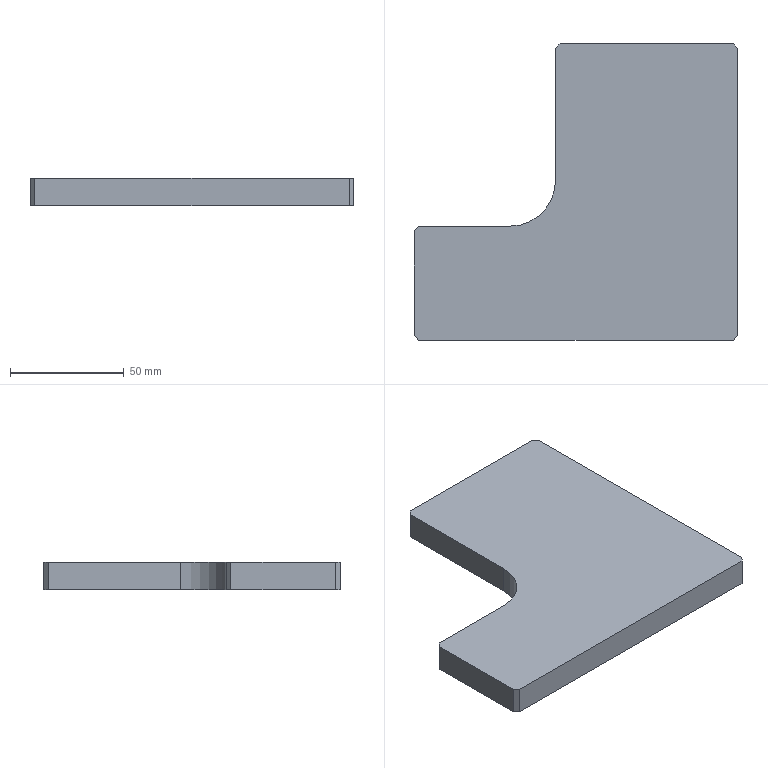Part | STEP file | 001-005-Shaft threading fixture cylinder mounting plate | 1 solid | 18 faces | box 142 x 130 x 12 mm | volume 162627 mm3 | plane 13 | cylinder 3 | cone 2 | commonest cylinder face diameters 4.2 x2 40 x1
STEP:
#1=CARTESIAN_POINT('',(0.,0.,0.));
#2=DIRECTION('',(0.,0.,1.));
#3=DIRECTION('',(1.,0.,0.));
#4=AXIS2_PLACEMENT_3D('',#1,#2,#3);
#5=CARTESIAN_POINT('',(31.,45.,8.1));
#6=VERTEX_POINT('',#5);
#7=CARTESIAN_POINT('',(31.,65.,8.1));
#8=VERTEX_POINT('',#7);
#9=CARTESIAN_POINT('',(31.,65.,8.1));
#10=DIRECTION('',(0.,1.,0.));
#11=VECTOR('',#10,1.);
#12=LINE('',#9,#11);
#13=CARTESIAN_POINT('',(31.,65.,6.));
#14=DIRECTION('',(0.,1.,0.));
#15=DIRECTION('',(0.,0.,1.));
#16=AXIS2_PLACEMENT_3D('',#13,#14,#15);
#17=CYLINDRICAL_SURFACE('',#16,2.1);
#18=CARTESIAN_POINT('',(6.283,0.));
#19=DIRECTION('',(0.,1.));
#20=VECTOR('',#19,1.);
#21=LINE('',#18,#20);
#22=(GEOMETRIC_REPRESENTATION_CONTEXT(2)PARAMETRIC_REPRESENTATION_CONTEXT()REPRESENTATION_CONTEXT('',''));
#23=DEFINITIONAL_REPRESENTATION('',(#21),#22);
#24=PCURVE('',#17,#23);
#25=CARTESIAN_POINT('',(31.,65.,6.));
#26=DIRECTION('',(0.,1.,0.));
#27=DIRECTION('',(0.,0.,1.));
#28=AXIS2_PLACEMENT_3D('',#25,#26,#27);
#29=CYLINDRICAL_SURFACE('',#28,2.1);
#30=CARTESIAN_POINT('',(0.,0.));
#31=DIRECTION('',(0.,1.));
#32=VECTOR('',#31,1.);
#33=LINE('',#30,#32);
#34=(GEOMETRIC_REPRESENTATION_CONTEXT(2)PARAMETRIC_REPRESENTATION_CONTEXT()REPRESENTATION_CONTEXT('',''));
#35=DEFINITIONAL_REPRESENTATION('',(#33),#34);
#36=PCURVE('',#29,#35);
#37=SURFACE_CURVE('',#12,(#24,#36),.PCURVE_S1.);
#38=EDGE_CURVE('',#6,#8,#37,.T.);
#39=ORIENTED_EDGE('',*,*,#38,.T.);
#40=CARTESIAN_POINT('',(31.,65.,3.9));
#41=VERTEX_POINT('',#40);
#42=CARTESIAN_POINT('',(31.,65.,6.));
#43=DIRECTION('',(0.,1.,0.));
#44=DIRECTION('',(0.,0.,1.));
#45=AXIS2_PLACEMENT_3D('',#42,#43,#44);
#46=CIRCLE('',#45,2.1);
#47=CARTESIAN_POINT('',(0.,0.));
#48=DIRECTION('',(1.,0.));
#49=VECTOR('',#48,1.);
#50=LINE('',#47,#49);
#51=(GEOMETRIC_REPRESENTATION_CONTEXT(2)PARAMETRIC_REPRESENTATION_CONTEXT()REPRESENTATION_CONTEXT('',''));
#52=DEFINITIONAL_REPRESENTATION('',(#50),#51);
#53=PCURVE('',#17,#52);
#54=CARTESIAN_POINT('',(-71.,65.,12.));
#55=DIRECTION('',(0.,-1.,0.));
#56=DIRECTION('',(1.,0.,0.));
#57=AXIS2_PLACEMENT_3D('',#54,#55,#56);
#58=PLANE('',#57);
#59=CARTESIAN_POINT('',(102.,-3.9));
#60=CARTESIAN_POINT('',(105.637,-3.9));
#61=CARTESIAN_POINT('',(103.819,-7.05));
#62=CARTESIAN_POINT('',(102.,-10.2));
#63=CARTESIAN_POINT('',(100.181,-7.05));
#64=CARTESIAN_POINT('',(98.363,-3.9));
#65=CARTESIAN_POINT('',(102.,-3.9));
#66=(BOUNDED_CURVE()B_SPLINE_CURVE(2,(#59,#60,#61,#62,#63,#64,#65),.UNSPECIFIED.,.T.,.F.)B_SPLINE_CURVE_WITH_KNOTS((1,2,2,2,2,1),(-2.094,0.,2.094,4.189,6.283,8.378),.UNSPECIFIED.)CURVE()GEOMETRIC_REPRESENTATION_ITEM()RATIONAL_B_SPLINE_CURVE((1.,0.5,1.,0.5,1.,0.5,1.))REPRESENTATION_ITEM(''));
#67=(GEOMETRIC_REPRESENTATION_CONTEXT(2)PARAMETRIC_REPRESENTATION_CONTEXT()REPRESENTATION_CONTEXT('',''));
#68=DEFINITIONAL_REPRESENTATION('',(#66),#67);
#69=PCURVE('',#58,#68);
#70=SURFACE_CURVE('',#46,(#53,#69),.PCURVE_S1.);
#71=EDGE_CURVE('',#41,#8,#70,.T.);
#72=ORIENTED_EDGE('',*,*,#71,.F.);
#73=CARTESIAN_POINT('',(31.,45.,3.9));
#74=VERTEX_POINT('',#73);
#75=CARTESIAN_POINT('',(31.,65.,3.9));
#76=DIRECTION('',(0.,1.,0.));
#77=VECTOR('',#76,1.);
#78=LINE('',#75,#77);
#79=CARTESIAN_POINT('',(3.142,0.));
#80=DIRECTION('',(0.,1.));
#81=VECTOR('',#80,1.);
#82=LINE('',#79,#81);
#83=(GEOMETRIC_REPRESENTATION_CONTEXT(2)PARAMETRIC_REPRESENTATION_CONTEXT()REPRESENTATION_CONTEXT('',''));
#84=DEFINITIONAL_REPRESENTATION('',(#82),#83);
#85=PCURVE('',#17,#84);
#86=CARTESIAN_POINT('',(3.142,0.));
#87=DIRECTION('',(0.,1.));
#88=VECTOR('',#87,1.);
#89=LINE('',#86,#88);
#90=(GEOMETRIC_REPRESENTATION_CONTEXT(2)PARAMETRIC_REPRESENTATION_CONTEXT()REPRESENTATION_CONTEXT('',''));
#91=DEFINITIONAL_REPRESENTATION('',(#89),#90);
#92=PCURVE('',#29,#91);
#93=SURFACE_CURVE('',#78,(#85,#92),.PCURVE_S1.);
#94=EDGE_CURVE('',#74,#41,#93,.T.);
#95=ORIENTED_EDGE('',*,*,#94,.F.);
#96=CARTESIAN_POINT('',(31.,45.,6.));
#97=DIRECTION('',(0.,1.,0.));
#98=DIRECTION('',(0.,0.,1.));
#99=AXIS2_PLACEMENT_3D('',#96,#97,#98);
#100=CIRCLE('',#99,2.1);
#101=CARTESIAN_POINT('',(0.,-20.));
#102=DIRECTION('',(1.,0.));
#103=VECTOR('',#102,1.);
#104=LINE('',#101,#103);
#105=(GEOMETRIC_REPRESENTATION_CONTEXT(2)PARAMETRIC_REPRESENTATION_CONTEXT()REPRESENTATION_CONTEXT('',''));
#106=DEFINITIONAL_REPRESENTATION('',(#104),#105);
#107=PCURVE('',#17,#106);
#108=CARTESIAN_POINT('',(31.,45.,6.));
#109=DIRECTION('',(0.,1.,0.));
#110=DIRECTION('',(0.,0.,1.));
#111=AXIS2_PLACEMENT_3D('',#108,#109,#110);
#112=CONICAL_SURFACE('',#111,2.1,1.03);
#113=CARTESIAN_POINT('',(0.,0.));
#114=DIRECTION('',(1.,0.));
#115=VECTOR('',#114,1.);
#116=LINE('',#113,#115);
#117=(GEOMETRIC_REPRESENTATION_CONTEXT(2)PARAMETRIC_REPRESENTATION_CONTEXT()REPRESENTATION_CONTEXT('',''));
#118=DEFINITIONAL_REPRESENTATION('',(#116),#117);
#119=PCURVE('',#112,#118);
#120=SURFACE_CURVE('',#100,(#107,#119),.PCURVE_S1.);
#121=EDGE_CURVE('',#74,#6,#120,.T.);
#122=ORIENTED_EDGE('',*,*,#121,.T.);
#123=EDGE_LOOP('',(#39,#72,#95,#122));
#124=FACE_BOUND('',#123,.F.);
#125=ADVANCED_FACE('',(#124),#17,.F.);
#126=ORIENTED_EDGE('',*,*,#121,.F.);
#127=CARTESIAN_POINT('',(31.,43.738,6.));
#128=VERTEX_POINT('',#127);
#129=CARTESIAN_POINT('',(31.,45.,3.9));
#130=DIRECTION('',(0.,0.515,-0.8572));
#131=VECTOR('',#130,1.);
#132=LINE('',#129,#131);
#133=CARTESIAN_POINT('',(3.142,-1.262));
#134=CARTESIAN_POINT('',(3.142,-1.243));
#135=CARTESIAN_POINT('',(3.142,-1.204));
#136=CARTESIAN_POINT('',(3.142,-1.147));
#137=CARTESIAN_POINT('',(3.142,-1.09));
#138=CARTESIAN_POINT('',(3.142,-1.032));
#139=CARTESIAN_POINT('',(3.142,-0.975));
#140=CARTESIAN_POINT('',(3.142,-0.9177));
#141=CARTESIAN_POINT('',(3.142,-0.8603));
#142=CARTESIAN_POINT('',(3.142,-0.803));
#143=CARTESIAN_POINT('',(3.142,-0.7456));
#144=CARTESIAN_POINT('',(3.142,-0.6883));
#145=CARTESIAN_POINT('',(3.142,-0.6309));
#146=CARTESIAN_POINT('',(3.142,-0.5735));
#147=CARTESIAN_POINT('',(3.142,-0.5162));
#148=CARTESIAN_POINT('',(3.142,-0.4588));
#149=CARTESIAN_POINT('',(3.142,-0.4015));
#150=CARTESIAN_POINT('',(3.142,-0.3441));
#151=CARTESIAN_POINT('',(3.142,-0.2868));
#152=CARTESIAN_POINT('',(3.142,-0.2294));
#153=CARTESIAN_POINT('',(3.142,-0.1721));
#154=CARTESIAN_POINT('',(3.142,-0.1147));
#155=CARTESIAN_POINT('',(3.142,-0.05735));
#156=CARTESIAN_POINT('',(3.142,-0.01912));
#157=CARTESIAN_POINT('',(3.142,0.));
#158=B_SPLINE_CURVE_WITH_KNOTS('',3,(#133,#134,#135,#136,#137,#138,#139,#140,#141,#142,#143,#144,#145,#146,#147,#148,#149,#150,#151,#152,#153,#154,#155,#156,#157),.UNSPECIFIED.,.F.,.F.,(4,1,1,1,1,1,1,1,1,1,1,1,1,1,1,1,1,1,1,1,1,1,4),(-2.45,-2.339,-2.227,-2.116,-2.004,-1.893,-1.782,-1.67,-1.559,-1.448,-1.336,-1.225,-1.114,-1.002,-0.8909,-0.7795,-0.6682,-0.5568,-0.4454,-0.3341,-0.2227,-0.1114,0.),.QUASI_UNIFORM_KNOTS.);
#159=(GEOMETRIC_REPRESENTATION_CONTEXT(2)PARAMETRIC_REPRESENTATION_CONTEXT()REPRESENTATION_CONTEXT('',''));
#160=DEFINITIONAL_REPRESENTATION('',(#158),#159);
#161=PCURVE('',#112,#160);
#162=CARTESIAN_POINT('',(31.,45.,6.));
#163=DIRECTION('',(0.,1.,0.));
#164=DIRECTION('',(0.,0.,1.));
#165=AXIS2_PLACEMENT_3D('',#162,#163,#164);
#166=CONICAL_SURFACE('',#165,2.1,1.03);
#167=CARTESIAN_POINT('',(3.142,-1.262));
#168=CARTESIAN_POINT('',(3.142,-1.243));
#169=CARTESIAN_POINT('',(3.142,-1.204));
#170=CARTESIAN_POINT('',(3.142,-1.147));
#171=CARTESIAN_POINT('',(3.142,-1.09));
#172=CARTESIAN_POINT('',(3.142,-1.032));
#173=CARTESIAN_POINT('',(3.142,-0.975));
#174=CARTESIAN_POINT('',(3.142,-0.9177));
#175=CARTESIAN_POINT('',(3.142,-0.8603));
#176=CARTESIAN_POINT('',(3.142,-0.803));
#177=CARTESIAN_POINT('',(3.142,-0.7456));
#178=CARTESIAN_POINT('',(3.142,-0.6883));
#179=CARTESIAN_POINT('',(3.142,-0.6309));
#180=CARTESIAN_POINT('',(3.142,-0.5735));
#181=CARTESIAN_POINT('',(3.142,-0.5162));
#182=CARTESIAN_POINT('',(3.142,-0.4588));
#183=CARTESIAN_POINT('',(3.142,-0.4015));
#184=CARTESIAN_POINT('',(3.142,-0.3441));
#185=CARTESIAN_POINT('',(3.142,-0.2868));
#186=CARTESIAN_POINT('',(3.142,-0.2294));
#187=CARTESIAN_POINT('',(3.142,-0.1721));
#188=CARTESIAN_POINT('',(3.142,-0.1147));
#189=CARTESIAN_POINT('',(3.142,-0.05735));
#190=CARTESIAN_POINT('',(3.142,-0.01912));
#191=CARTESIAN_POINT('',(3.142,0.));
#192=B_SPLINE_CURVE_WITH_KNOTS('',3,(#167,#168,#169,#170,#171,#172,#173,#174,#175,#176,#177,#178,#179,#180,#181,#182,#183,#184,#185,#186,#187,#188,#189,#190,#191),.UNSPECIFIED.,.F.,.F.,(4,1,1,1,1,1,1,1,1,1,1,1,1,1,1,1,1,1,1,1,1,1,4),(-2.45,-2.339,-2.227,-2.116,-2.004,-1.893,-1.782,-1.67,-1.559,-1.448,-1.336,-1.225,-1.114,-1.002,-0.8909,-0.7795,-0.6682,-0.5568,-0.4454,-0.3341,-0.2227,-0.1114,0.),.QUASI_UNIFORM_KNOTS.);
#193=(GEOMETRIC_REPRESENTATION_CONTEXT(2)PARAMETRIC_REPRESENTATION_CONTEXT()REPRESENTATION_CONTEXT('',''));
#194=DEFINITIONAL_REPRESENTATION('',(#192),#193);
#195=PCURVE('',#166,#194);
#196=SURFACE_CURVE('',#132,(#161,#195),.PCURVE_S1.);
#197=EDGE_CURVE('',#128,#74,#196,.T.);
#198=ORIENTED_EDGE('',*,*,#197,.F.);
#199=CARTESIAN_POINT('',(31.,45.,8.1));
#200=DIRECTION('',(0.,0.515,0.8572));
#201=VECTOR('',#200,1.);
#202=LINE('',#199,#201);
#203=CARTESIAN_POINT('',(6.283,-1.262));
#204=CARTESIAN_POINT('',(6.283,-1.243));
#205=CARTESIAN_POINT('',(6.283,-1.204));
#206=CARTESIAN_POINT('',(6.283,-1.147));
#207=CARTESIAN_POINT('',(6.283,-1.09));
#208=CARTESIAN_POINT('',(6.283,-1.032));
#209=CARTESIAN_POINT('',(6.283,-0.975));
#210=CARTESIAN_POINT('',(6.283,-0.9177));
#211=CARTESIAN_POINT('',(6.283,-0.8603));
#212=CARTESIAN_POINT('',(6.283,-0.803));
#213=CARTESIAN_POINT('',(6.283,-0.7456));
#214=CARTESIAN_POINT('',(6.283,-0.6883));
#215=CARTESIAN_POINT('',(6.283,-0.6309));
#216=CARTESIAN_POINT('',(6.283,-0.5735));
#217=CARTESIAN_POINT('',(6.283,-0.5162));
#218=CARTESIAN_POINT('',(6.283,-0.4588));
#219=CARTESIAN_POINT('',(6.283,-0.4015));
#220=CARTESIAN_POINT('',(6.283,-0.3441));
#221=CARTESIAN_POINT('',(6.283,-0.2868));
#222=CARTESIAN_POINT('',(6.283,-0.2294));
#223=CARTESIAN_POINT('',(6.283,-0.1721));
#224=CARTESIAN_POINT('',(6.283,-0.1147));
#225=CARTESIAN_POINT('',(6.283,-0.05735));
#226=CARTESIAN_POINT('',(6.283,-0.01912));
#227=CARTESIAN_POINT('',(6.283,0.));
#228=B_SPLINE_CURVE_WITH_KNOTS('',3,(#203,#204,#205,#206,#207,#208,#209,#210,#211,#212,#213,#214,#215,#216,#217,#218,#219,#220,#221,#222,#223,#224,#225,#226,#227),.UNSPECIFIED.,.F.,.F.,(4,1,1,1,1,1,1,1,1,1,1,1,1,1,1,1,1,1,1,1,1,1,4),(-2.45,-2.339,-2.227,-2.116,-2.004,-1.893,-1.782,-1.67,-1.559,-1.448,-1.336,-1.225,-1.114,-1.002,-0.8909,-0.7795,-0.6682,-0.5568,-0.4454,-0.3341,-0.2227,-0.1114,0.),.UNSPECIFIED.);
#229=(GEOMETRIC_REPRESENTATION_CONTEXT(2)PARAMETRIC_REPRESENTATION_CONTEXT()REPRESENTATION_CONTEXT('',''));
#230=DEFINITIONAL_REPRESENTATION('',(#228),#229);
#231=PCURVE('',#112,#230);
#232=CARTESIAN_POINT('',(0.,-1.262));
#233=CARTESIAN_POINT('',(0.,-1.243));
#234=CARTESIAN_POINT('',(0.,-1.204));
#235=CARTESIAN_POINT('',(0.,-1.147));
#236=CARTESIAN_POINT('',(0.,-1.09));
#237=CARTESIAN_POINT('',(0.,-1.032));
#238=CARTESIAN_POINT('',(0.,-0.975));
#239=CARTESIAN_POINT('',(0.,-0.9177));
#240=CARTESIAN_POINT('',(0.,-0.8603));
#241=CARTESIAN_POINT('',(0.,-0.803));
#242=CARTESIAN_POINT('',(0.,-0.7456));
#243=CARTESIAN_POINT('',(0.,-0.6883));
#244=CARTESIAN_POINT('',(0.,-0.6309));
#245=CARTESIAN_POINT('',(0.,-0.5735));
#246=CARTESIAN_POINT('',(0.,-0.5162));
#247=CARTESIAN_POINT('',(0.,-0.4588));
#248=CARTESIAN_POINT('',(0.,-0.4015));
#249=CARTESIAN_POINT('',(0.,-0.3441));
#250=CARTESIAN_POINT('',(0.,-0.2868));
#251=CARTESIAN_POINT('',(0.,-0.2294));
#252=CARTESIAN_POINT('',(0.,-0.1721));
#253=CARTESIAN_POINT('',(0.,-0.1147));
#254=CARTESIAN_POINT('',(0.,-0.05735));
#255=CARTESIAN_POINT('',(0.,-0.01912));
#256=CARTESIAN_POINT('',(0.,0.));
#257=B_SPLINE_CURVE_WITH_KNOTS('',3,(#232,#233,#234,#235,#236,#237,#238,#239,#240,#241,#242,#243,#244,#245,#246,#247,#248,#249,#250,#251,#252,#253,#254,#255,#256),.UNSPECIFIED.,.F.,.F.,(4,1,1,1,1,1,1,1,1,1,1,1,1,1,1,1,1,1,1,1,1,1,4),(-2.45,-2.339,-2.227,-2.116,-2.004,-1.893,-1.782,-1.67,-1.559,-1.448,-1.336,-1.225,-1.114,-1.002,-0.8909,-0.7795,-0.6682,-0.5568,-0.4454,-0.3341,-0.2227,-0.1114,0.),.UNSPECIFIED.);
#258=(GEOMETRIC_REPRESENTATION_CONTEXT(2)PARAMETRIC_REPRESENTATION_CONTEXT()REPRESENTATION_CONTEXT('',''));
#259=DEFINITIONAL_REPRESENTATION('',(#257),#258);
#260=PCURVE('',#166,#259);
#261=SURFACE_CURVE('',#202,(#231,#260),.PCURVE_S1.);
#262=EDGE_CURVE('',#128,#6,#261,.T.);
#263=ORIENTED_EDGE('',*,*,#262,.T.);
#264=EDGE_LOOP('',(#126,#198,#263));
#265=FACE_BOUND('',#264,.F.);
#266=ADVANCED_FACE('',(#265),#112,.F.);
#267=CARTESIAN_POINT('',(31.,65.,6.));
#268=DIRECTION('',(0.,1.,0.));
#269=DIRECTION('',(0.,0.,1.));
#270=AXIS2_PLACEMENT_3D('',#267,#268,#269);
#271=CIRCLE('',#270,2.1);
#272=CARTESIAN_POINT('',(102.,-3.9));
#273=CARTESIAN_POINT('',(105.637,-3.9));
#274=CARTESIAN_POINT('',(103.819,-7.05));
#275=CARTESIAN_POINT('',(102.,-10.2));
#276=CARTESIAN_POINT('',(100.181,-7.05));
#277=CARTESIAN_POINT('',(98.363,-3.9));
#278=CARTESIAN_POINT('',(102.,-3.9));
#279=(BOUNDED_CURVE()B_SPLINE_CURVE(2,(#272,#273,#274,#275,#276,#277,#278),.UNSPECIFIED.,.T.,.F.)B_SPLINE_CURVE_WITH_KNOTS((1,2,2,2,2,1),(-2.094,0.,2.094,4.189,6.283,8.378),.UNSPECIFIED.)CURVE()GEOMETRIC_REPRESENTATION_ITEM()RATIONAL_B_SPLINE_CURVE((1.,0.5,1.,0.5,1.,0.5,1.))REPRESENTATION_ITEM(''));
#280=(GEOMETRIC_REPRESENTATION_CONTEXT(2)PARAMETRIC_REPRESENTATION_CONTEXT()REPRESENTATION_CONTEXT('',''));
#281=DEFINITIONAL_REPRESENTATION('',(#279),#280);
#282=PCURVE('',#58,#281);
#283=CARTESIAN_POINT('',(0.,0.));
#284=DIRECTION('',(1.,0.));
#285=VECTOR('',#284,1.);
#286=LINE('',#283,#285);
#287=(GEOMETRIC_REPRESENTATION_CONTEXT(2)PARAMETRIC_REPRESENTATION_CONTEXT()REPRESENTATION_CONTEXT('',''));
#288=DEFINITIONAL_REPRESENTATION('',(#286),#287);
#289=PCURVE('',#29,#288);
#290=SURFACE_CURVE('',#271,(#282,#289),.PCURVE_S1.);
#291=EDGE_CURVE('',#8,#41,#290,.T.);
#292=ORIENTED_EDGE('',*,*,#291,.F.);
#293=ORIENTED_EDGE('',*,*,#71,.F.);
#294=EDGE_LOOP('',(#292,#293));
#295=FACE_BOUND('',#294,.T.);
#296=CARTESIAN_POINT('',(69.,65.,0.));
#297=VERTEX_POINT('',#296);
#298=CARTESIAN_POINT('',(-7.,65.,0.));
#299=VERTEX_POINT('',#298);
#300=CARTESIAN_POINT('',(-71.,65.,0.));
#301=DIRECTION('',(-1.,0.,0.));
#302=VECTOR('',#301,1.);
#303=LINE('',#300,#302);
#304=CARTESIAN_POINT('',(0.,-12.));
#305=DIRECTION('',(-1.,0.));
#306=VECTOR('',#305,1.);
#307=LINE('',#304,#306);
#308=(GEOMETRIC_REPRESENTATION_CONTEXT(2)PARAMETRIC_REPRESENTATION_CONTEXT()REPRESENTATION_CONTEXT('',''));
#309=DEFINITIONAL_REPRESENTATION('',(#307),#308);
#310=PCURVE('',#58,#309);
#311=CARTESIAN_POINT('',(0.,0.,0.));
#312=DIRECTION('',(0.,0.,-1.));
#313=DIRECTION('',(-1.,0.,0.));
#314=AXIS2_PLACEMENT_3D('',#311,#312,#313);
#315=PLANE('',#314);
#316=CARTESIAN_POINT('',(71.,65.));
#317=DIRECTION('',(1.,0.));
#318=VECTOR('',#317,1.);
#319=LINE('',#316,#318);
#320=(GEOMETRIC_REPRESENTATION_CONTEXT(2)PARAMETRIC_REPRESENTATION_CONTEXT()REPRESENTATION_CONTEXT('',''));
#321=DEFINITIONAL_REPRESENTATION('',(#319),#320);
#322=PCURVE('',#315,#321);
#323=SURFACE_CURVE('',#303,(#310,#322),.PCURVE_S1.);
#324=EDGE_CURVE('',#297,#299,#323,.T.);
#325=ORIENTED_EDGE('',*,*,#324,.T.);
#326=CARTESIAN_POINT('',(-7.,65.,12.));
#327=VERTEX_POINT('',#326);
#328=CARTESIAN_POINT('',(-7.,65.,12.));
#329=DIRECTION('',(0.,0.,1.));
#330=VECTOR('',#329,1.);
#331=LINE('',#328,#330);
#332=CARTESIAN_POINT('',(64.,0.));
#333=DIRECTION('',(0.,1.));
#334=VECTOR('',#333,1.);
#335=LINE('',#332,#334);
#336=(GEOMETRIC_REPRESENTATION_CONTEXT(2)PARAMETRIC_REPRESENTATION_CONTEXT()REPRESENTATION_CONTEXT('',''));
#337=DEFINITIONAL_REPRESENTATION('',(#335),#336);
#338=PCURVE('',#58,#337);
#339=CARTESIAN_POINT('',(-9.,63.,12.));
#340=DIRECTION('',(-0.7071,0.7071,0.));
#341=DIRECTION('',(0.,0.,1.));
#342=AXIS2_PLACEMENT_3D('',#339,#340,#341);
#343=PLANE('',#342);
#344=CARTESIAN_POINT('',(0.,2.828));
#345=DIRECTION('',(1.,0.));
#346=VECTOR('',#345,1.);
#347=LINE('',#344,#346);
#348=(GEOMETRIC_REPRESENTATION_CONTEXT(2)PARAMETRIC_REPRESENTATION_CONTEXT()REPRESENTATION_CONTEXT('',''));
#349=DEFINITIONAL_REPRESENTATION('',(#347),#348);
#350=PCURVE('',#343,#349);
#351=SURFACE_CURVE('',#331,(#338,#350),.PCURVE_S1.);
#352=EDGE_CURVE('',#299,#327,#351,.T.);
#353=ORIENTED_EDGE('',*,*,#352,.T.);
#354=CARTESIAN_POINT('',(69.,65.,12.));
#355=VERTEX_POINT('',#354);
#356=CARTESIAN_POINT('',(-71.,65.,12.));
#357=DIRECTION('',(-1.,0.,0.));
#358=VECTOR('',#357,1.);
#359=LINE('',#356,#358);
#360=CARTESIAN_POINT('',(0.,0.));
#361=DIRECTION('',(-1.,0.));
#362=VECTOR('',#361,1.);
#363=LINE('',#360,#362);
#364=(GEOMETRIC_REPRESENTATION_CONTEXT(2)PARAMETRIC_REPRESENTATION_CONTEXT()REPRESENTATION_CONTEXT('',''));
#365=DEFINITIONAL_REPRESENTATION('',(#363),#364);
#366=PCURVE('',#58,#365);
#367=CARTESIAN_POINT('',(0.,0.,12.));
#368=DIRECTION('',(0.,0.,-1.));
#369=DIRECTION('',(-1.,0.,0.));
#370=AXIS2_PLACEMENT_3D('',#367,#368,#369);
#371=PLANE('',#370);
#372=CARTESIAN_POINT('',(71.,65.));
#373=DIRECTION('',(1.,0.));
#374=VECTOR('',#373,1.);
#375=LINE('',#372,#374);
#376=(GEOMETRIC_REPRESENTATION_CONTEXT(2)PARAMETRIC_REPRESENTATION_CONTEXT()REPRESENTATION_CONTEXT('',''));
#377=DEFINITIONAL_REPRESENTATION('',(#375),#376);
#378=PCURVE('',#371,#377);
#379=SURFACE_CURVE('',#359,(#366,#378),.PCURVE_S1.);
#380=EDGE_CURVE('',#355,#327,#379,.T.);
#381=ORIENTED_EDGE('',*,*,#380,.F.);
#382=CARTESIAN_POINT('',(69.,65.,12.));
#383=DIRECTION('',(0.,0.,-1.));
#384=VECTOR('',#383,1.);
#385=LINE('',#382,#384);
#386=CARTESIAN_POINT('',(140.,0.));
#387=DIRECTION('',(0.,-1.));
#388=VECTOR('',#387,1.);
#389=LINE('',#386,#388);
#390=(GEOMETRIC_REPRESENTATION_CONTEXT(2)PARAMETRIC_REPRESENTATION_CONTEXT()REPRESENTATION_CONTEXT('',''));
#391=DEFINITIONAL_REPRESENTATION('',(#389),#390);
#392=PCURVE('',#58,#391);
#393=CARTESIAN_POINT('',(69.,65.,12.));
#394=DIRECTION('',(-0.7071,-0.7071,0.));
#395=DIRECTION('',(0.,0.,-1.));
#396=AXIS2_PLACEMENT_3D('',#393,#394,#395);
#397=PLANE('',#396);
#398=CARTESIAN_POINT('',(0.,0.));
#399=DIRECTION('',(1.,0.));
#400=VECTOR('',#399,1.);
#401=LINE('',#398,#400);
#402=(GEOMETRIC_REPRESENTATION_CONTEXT(2)PARAMETRIC_REPRESENTATION_CONTEXT()REPRESENTATION_CONTEXT('',''));
#403=DEFINITIONAL_REPRESENTATION('',(#401),#402);
#404=PCURVE('',#397,#403);
#405=SURFACE_CURVE('',#385,(#392,#404),.PCURVE_S1.);
#406=EDGE_CURVE('',#355,#297,#405,.T.);
#407=ORIENTED_EDGE('',*,*,#406,.T.);
#408=EDGE_LOOP('',(#325,#353,#381,#407));
#409=FACE_BOUND('',#408,.T.);
#410=ADVANCED_FACE('',(#295,#409),#58,.F.);
#411=CARTESIAN_POINT('',(-71.,-17.,0.));
#412=VERTEX_POINT('',#411);
#413=CARTESIAN_POINT('',(-71.,-63.,0.));
#414=VERTEX_POINT('',#413);
#415=CARTESIAN_POINT('',(-71.,-65.,0.));
#416=DIRECTION('',(0.,-1.,0.));
#417=VECTOR('',#416,1.);
#418=LINE('',#415,#417);
#419=CARTESIAN_POINT('',(-71.,-65.,12.));
#420=DIRECTION('',(1.,0.,0.));
#421=DIRECTION('',(0.,0.,-1.));
#422=AXIS2_PLACEMENT_3D('',#419,#420,#421);
#423=PLANE('',#422);
#424=CARTESIAN_POINT('',(12.,0.));
#425=DIRECTION('',(0.,-1.));
#426=VECTOR('',#425,1.);
#427=LINE('',#424,#426);
#428=(GEOMETRIC_REPRESENTATION_CONTEXT(2)PARAMETRIC_REPRESENTATION_CONTEXT()REPRESENTATION_CONTEXT('',''));
#429=DEFINITIONAL_REPRESENTATION('',(#427),#428);
#430=PCURVE('',#423,#429);
#431=CARTESIAN_POINT('',(71.,-65.));
#432=DIRECTION('',(0.,-1.));
#433=VECTOR('',#432,1.);
#434=LINE('',#431,#433);
#435=(GEOMETRIC_REPRESENTATION_CONTEXT(2)PARAMETRIC_REPRESENTATION_CONTEXT()REPRESENTATION_CONTEXT('',''));
#436=DEFINITIONAL_REPRESENTATION('',(#434),#435);
#437=PCURVE('',#315,#436);
#438=SURFACE_CURVE('',#418,(#430,#437),.PCURVE_S1.);
#439=EDGE_CURVE('',#412,#414,#438,.T.);
#440=ORIENTED_EDGE('',*,*,#439,.T.);
#441=CARTESIAN_POINT('',(-71.,-63.,12.));
#442=VERTEX_POINT('',#441);
#443=CARTESIAN_POINT('',(-71.,-63.,12.));
#444=DIRECTION('',(0.,0.,1.));
#445=VECTOR('',#444,1.);
#446=LINE('',#443,#445);
#447=CARTESIAN_POINT('',(0.,2.));
#448=DIRECTION('',(-1.,0.));
#449=VECTOR('',#448,1.);
#450=LINE('',#447,#449);
#451=(GEOMETRIC_REPRESENTATION_CONTEXT(2)PARAMETRIC_REPRESENTATION_CONTEXT()REPRESENTATION_CONTEXT('',''));
#452=DEFINITIONAL_REPRESENTATION('',(#450),#451);
#453=PCURVE('',#423,#452);
#454=CARTESIAN_POINT('',(-69.,-65.,12.));
#455=DIRECTION('',(0.7071,0.7071,0.));
#456=DIRECTION('',(0.,0.,-1.));
#457=AXIS2_PLACEMENT_3D('',#454,#455,#456);
#458=PLANE('',#457);
#459=CARTESIAN_POINT('',(0.,2.828));
#460=DIRECTION('',(-1.,0.));
#461=VECTOR('',#460,1.);
#462=LINE('',#459,#461);
#463=(GEOMETRIC_REPRESENTATION_CONTEXT(2)PARAMETRIC_REPRESENTATION_CONTEXT()REPRESENTATION_CONTEXT('',''));
#464=DEFINITIONAL_REPRESENTATION('',(#462),#463);
#465=PCURVE('',#458,#464);
#466=SURFACE_CURVE('',#446,(#453,#465),.PCURVE_S1.);
#467=EDGE_CURVE('',#414,#442,#466,.T.);
#468=ORIENTED_EDGE('',*,*,#467,.T.);
#469=CARTESIAN_POINT('',(-71.,-17.,12.));
#470=VERTEX_POINT('',#469);
#471=CARTESIAN_POINT('',(-71.,-65.,12.));
#472=DIRECTION('',(0.,-1.,0.));
#473=VECTOR('',#472,1.);
#474=LINE('',#471,#473);
#475=CARTESIAN_POINT('',(0.,0.));
#476=DIRECTION('',(0.,-1.));
#477=VECTOR('',#476,1.);
#478=LINE('',#475,#477);
#479=(GEOMETRIC_REPRESENTATION_CONTEXT(2)PARAMETRIC_REPRESENTATION_CONTEXT()REPRESENTATION_CONTEXT('',''));
#480=DEFINITIONAL_REPRESENTATION('',(#478),#479);
#481=PCURVE('',#423,#480);
#482=CARTESIAN_POINT('',(71.,-65.));
#483=DIRECTION('',(0.,-1.));
#484=VECTOR('',#483,1.);
#485=LINE('',#482,#484);
#486=(GEOMETRIC_REPRESENTATION_CONTEXT(2)PARAMETRIC_REPRESENTATION_CONTEXT()REPRESENTATION_CONTEXT('',''));
#487=DEFINITIONAL_REPRESENTATION('',(#485),#486);
#488=PCURVE('',#371,#487);
#489=SURFACE_CURVE('',#474,(#481,#488),.PCURVE_S1.);
#490=EDGE_CURVE('',#470,#442,#489,.T.);
#491=ORIENTED_EDGE('',*,*,#490,.F.);
#492=CARTESIAN_POINT('',(-71.,-17.,0.));
#493=DIRECTION('',(0.,0.,-1.));
#494=VECTOR('',#493,1.);
#495=LINE('',#492,#494);
#496=CARTESIAN_POINT('',(12.,48.));
#497=DIRECTION('',(1.,0.));
#498=VECTOR('',#497,1.);
#499=LINE('',#496,#498);
#500=(GEOMETRIC_REPRESENTATION_CONTEXT(2)PARAMETRIC_REPRESENTATION_CONTEXT()REPRESENTATION_CONTEXT('',''));
#501=DEFINITIONAL_REPRESENTATION('',(#499),#500);
#502=PCURVE('',#423,#501);
#503=CARTESIAN_POINT('',(-71.,-17.,12.));
#504=DIRECTION('',(-0.7071,0.7071,0.));
#505=DIRECTION('',(0.,0.,1.));
#506=AXIS2_PLACEMENT_3D('',#503,#504,#505);
#507=PLANE('',#506);
#508=CARTESIAN_POINT('',(-12.,0.));
#509=DIRECTION('',(-1.,0.));
#510=VECTOR('',#509,1.);
#511=LINE('',#508,#510);
#512=(GEOMETRIC_REPRESENTATION_CONTEXT(2)PARAMETRIC_REPRESENTATION_CONTEXT()REPRESENTATION_CONTEXT('',''));
#513=DEFINITIONAL_REPRESENTATION('',(#511),#512);
#514=PCURVE('',#507,#513);
#515=SURFACE_CURVE('',#495,(#502,#514),.PCURVE_S1.);
#516=EDGE_CURVE('',#470,#412,#515,.T.);
#517=ORIENTED_EDGE('',*,*,#516,.T.);
#518=EDGE_LOOP('',(#440,#468,#491,#517));
#519=FACE_BOUND('',#518,.T.);
#520=ADVANCED_FACE('',(#519),#423,.F.);
#521=ORIENTED_EDGE('',*,*,#380,.T.);
#522=CARTESIAN_POINT('',(-9.,63.,12.));
#523=VERTEX_POINT('',#522);
#524=CARTESIAN_POINT('',(-9.,63.,12.));
#525=DIRECTION('',(-0.7071,-0.7071,0.));
#526=VECTOR('',#525,1.);
#527=LINE('',#524,#526);
#528=CARTESIAN_POINT('',(9.,63.));
#529=DIRECTION('',(0.7071,-0.7071));
#530=VECTOR('',#529,1.);
#531=LINE('',#528,#530);
#532=(GEOMETRIC_REPRESENTATION_CONTEXT(2)PARAMETRIC_REPRESENTATION_CONTEXT()REPRESENTATION_CONTEXT('',''));
#533=DEFINITIONAL_REPRESENTATION('',(#531),#532);
#534=PCURVE('',#371,#533);
#535=CARTESIAN_POINT('',(0.,0.));
#536=DIRECTION('',(0.,-1.));
#537=VECTOR('',#536,1.);
#538=LINE('',#535,#537);
#539=(GEOMETRIC_REPRESENTATION_CONTEXT(2)PARAMETRIC_REPRESENTATION_CONTEXT()REPRESENTATION_CONTEXT('',''));
#540=DEFINITIONAL_REPRESENTATION('',(#538),#539);
#541=PCURVE('',#343,#540);
#542=SURFACE_CURVE('',#527,(#534,#541),.PCURVE_S1.);
#543=EDGE_CURVE('',#327,#523,#542,.T.);
#544=ORIENTED_EDGE('',*,*,#543,.T.);
#545=CARTESIAN_POINT('',(-9.,5.,12.));
#546=VERTEX_POINT('',#545);
#547=CARTESIAN_POINT('',(-9.,65.,12.));
#548=DIRECTION('',(0.,1.,0.));
#549=VECTOR('',#548,1.);
#550=LINE('',#547,#549);
#551=CARTESIAN_POINT('',(9.,65.));
#552=DIRECTION('',(0.,1.));
#553=VECTOR('',#552,1.);
#554=LINE('',#551,#553);
#555=(GEOMETRIC_REPRESENTATION_CONTEXT(2)PARAMETRIC_REPRESENTATION_CONTEXT()REPRESENTATION_CONTEXT('',''));
#556=DEFINITIONAL_REPRESENTATION('',(#554),#555);
#557=PCURVE('',#371,#556);
#558=CARTESIAN_POINT('',(-9.,65.,12.));
#559=DIRECTION('',(-1.,0.,0.));
#560=DIRECTION('',(0.,0.,1.));
#561=AXIS2_PLACEMENT_3D('',#558,#559,#560);
#562=PLANE('',#561);
#563=CARTESIAN_POINT('',(0.,0.));
#564=DIRECTION('',(0.,1.));
#565=VECTOR('',#564,1.);
#566=LINE('',#563,#565);
#567=(GEOMETRIC_REPRESENTATION_CONTEXT(2)PARAMETRIC_REPRESENTATION_CONTEXT()REPRESENTATION_CONTEXT('',''));
#568=DEFINITIONAL_REPRESENTATION('',(#566),#567);
#569=PCURVE('',#562,#568);
#570=SURFACE_CURVE('',#550,(#557,#569),.PCURVE_S1.);
#571=EDGE_CURVE('',#546,#523,#570,.T.);
#572=ORIENTED_EDGE('',*,*,#571,.F.);
#573=CARTESIAN_POINT('',(-29.,-15.,12.));
#574=VERTEX_POINT('',#573);
#575=CARTESIAN_POINT('',(-29.,5.,12.));
#576=DIRECTION('',(0.,0.,-1.));
#577=DIRECTION('',(-1.,0.,0.));
#578=AXIS2_PLACEMENT_3D('',#575,#576,#577);
#579=CIRCLE('',#578,20.);
#580=CARTESIAN_POINT('',(29.,5.));
#581=DIRECTION('',(1.,0.));
#582=AXIS2_PLACEMENT_2D('',#580,#581);
#583=CIRCLE('',#582,20.);
#584=(GEOMETRIC_REPRESENTATION_CONTEXT(2)PARAMETRIC_REPRESENTATION_CONTEXT()REPRESENTATION_CONTEXT('',''));
#585=DEFINITIONAL_REPRESENTATION('',(#583),#584);
#586=PCURVE('',#371,#585);
#587=CARTESIAN_POINT('',(-29.,5.,12.));
#588=DIRECTION('',(0.,0.,1.));
#589=DIRECTION('',(1.,0.,0.));
#590=AXIS2_PLACEMENT_3D('',#587,#588,#589);
#591=CYLINDRICAL_SURFACE('',#590,20.);
#592=CARTESIAN_POINT('',(9.425,0.));
#593=DIRECTION('',(-1.,0.));
#594=VECTOR('',#593,1.);
#595=LINE('',#592,#594);
#596=(GEOMETRIC_REPRESENTATION_CONTEXT(2)PARAMETRIC_REPRESENTATION_CONTEXT()REPRESENTATION_CONTEXT('',''));
#597=DEFINITIONAL_REPRESENTATION('',(#595),#596);
#598=PCURVE('',#591,#597);
#599=SURFACE_CURVE('',#579,(#586,#598),.PCURVE_S1.);
#600=EDGE_CURVE('',#546,#574,#599,.T.);
#601=ORIENTED_EDGE('',*,*,#600,.T.);
#602=CARTESIAN_POINT('',(-69.,-15.,12.));
#603=VERTEX_POINT('',#602);
#604=CARTESIAN_POINT('',(-71.,-15.,12.));
#605=DIRECTION('',(1.,0.,0.));
#606=VECTOR('',#605,1.);
#607=LINE('',#604,#606);
#608=CARTESIAN_POINT('',(71.,-15.));
#609=DIRECTION('',(-1.,0.));
#610=VECTOR('',#609,1.);
#611=LINE('',#608,#610);
#612=(GEOMETRIC_REPRESENTATION_CONTEXT(2)PARAMETRIC_REPRESENTATION_CONTEXT()REPRESENTATION_CONTEXT('',''));
#613=DEFINITIONAL_REPRESENTATION('',(#611),#612);
#614=PCURVE('',#371,#613);
#615=CARTESIAN_POINT('',(-71.,-15.,12.));
#616=DIRECTION('',(0.,1.,0.));
#617=DIRECTION('',(0.,0.,1.));
#618=AXIS2_PLACEMENT_3D('',#615,#616,#617);
#619=PLANE('',#618);
#620=CARTESIAN_POINT('',(0.,0.));
#621=DIRECTION('',(0.,1.));
#622=VECTOR('',#621,1.);
#623=LINE('',#620,#622);
#624=(GEOMETRIC_REPRESENTATION_CONTEXT(2)PARAMETRIC_REPRESENTATION_CONTEXT()REPRESENTATION_CONTEXT('',''));
#625=DEFINITIONAL_REPRESENTATION('',(#623),#624);
#626=PCURVE('',#619,#625);
#627=SURFACE_CURVE('',#607,(#614,#626),.PCURVE_S1.);
#628=EDGE_CURVE('',#603,#574,#627,.T.);
#629=ORIENTED_EDGE('',*,*,#628,.F.);
#630=CARTESIAN_POINT('',(-71.,-17.,12.));
#631=DIRECTION('',(-0.7071,-0.7071,0.));
#632=VECTOR('',#631,1.);
#633=LINE('',#630,#632);
#634=CARTESIAN_POINT('',(71.,-17.));
#635=DIRECTION('',(0.7071,-0.7071));
#636=VECTOR('',#635,1.);
#637=LINE('',#634,#636);
#638=(GEOMETRIC_REPRESENTATION_CONTEXT(2)PARAMETRIC_REPRESENTATION_CONTEXT()REPRESENTATION_CONTEXT('',''));
#639=DEFINITIONAL_REPRESENTATION('',(#637),#638);
#640=PCURVE('',#371,#639);
#641=CARTESIAN_POINT('',(0.,0.));
#642=DIRECTION('',(0.,-1.));
#643=VECTOR('',#642,1.);
#644=LINE('',#641,#643);
#645=(GEOMETRIC_REPRESENTATION_CONTEXT(2)PARAMETRIC_REPRESENTATION_CONTEXT()REPRESENTATION_CONTEXT('',''));
#646=DEFINITIONAL_REPRESENTATION('',(#644),#645);
#647=PCURVE('',#507,#646);
#648=SURFACE_CURVE('',#633,(#640,#647),.PCURVE_S1.);
#649=EDGE_CURVE('',#603,#470,#648,.T.);
#650=ORIENTED_EDGE('',*,*,#649,.T.);
#651=ORIENTED_EDGE('',*,*,#490,.T.);
#652=CARTESIAN_POINT('',(-69.,-65.,12.));
#653=VERTEX_POINT('',#652);
#654=CARTESIAN_POINT('',(-69.,-65.,12.));
#655=DIRECTION('',(0.7071,-0.7071,0.));
#656=VECTOR('',#655,1.);
#657=LINE('',#654,#656);
#658=CARTESIAN_POINT('',(69.,-65.));
#659=DIRECTION('',(-0.7071,-0.7071));
#660=VECTOR('',#659,1.);
#661=LINE('',#658,#660);
#662=(GEOMETRIC_REPRESENTATION_CONTEXT(2)PARAMETRIC_REPRESENTATION_CONTEXT()REPRESENTATION_CONTEXT('',''));
#663=DEFINITIONAL_REPRESENTATION('',(#661),#662);
#664=PCURVE('',#371,#663);
#665=CARTESIAN_POINT('',(0.,0.));
#666=DIRECTION('',(0.,-1.));
#667=VECTOR('',#666,1.);
#668=LINE('',#665,#667);
#669=(GEOMETRIC_REPRESENTATION_CONTEXT(2)PARAMETRIC_REPRESENTATION_CONTEXT()REPRESENTATION_CONTEXT('',''));
#670=DEFINITIONAL_REPRESENTATION('',(#668),#669);
#671=PCURVE('',#458,#670);
#672=SURFACE_CURVE('',#657,(#664,#671),.PCURVE_S1.);
#673=EDGE_CURVE('',#442,#653,#672,.T.);
#674=ORIENTED_EDGE('',*,*,#673,.T.);
#675=CARTESIAN_POINT('',(69.,-65.,12.));
#676=VERTEX_POINT('',#675);
#677=CARTESIAN_POINT('',(-71.,-65.,12.));
#678=DIRECTION('',(1.,0.,0.));
#679=VECTOR('',#678,1.);
#680=LINE('',#677,#679);
#681=CARTESIAN_POINT('',(71.,-65.));
#682=DIRECTION('',(-1.,0.));
#683=VECTOR('',#682,1.);
#684=LINE('',#681,#683);
#685=(GEOMETRIC_REPRESENTATION_CONTEXT(2)PARAMETRIC_REPRESENTATION_CONTEXT()REPRESENTATION_CONTEXT('',''));
#686=DEFINITIONAL_REPRESENTATION('',(#684),#685);
#687=PCURVE('',#371,#686);
#688=CARTESIAN_POINT('',(-71.,-65.,12.));
#689=DIRECTION('',(0.,1.,0.));
#690=DIRECTION('',(0.,0.,1.));
#691=AXIS2_PLACEMENT_3D('',#688,#689,#690);
#692=PLANE('',#691);
#693=CARTESIAN_POINT('',(0.,0.));
#694=DIRECTION('',(0.,1.));
#695=VECTOR('',#694,1.);
#696=LINE('',#693,#695);
#697=(GEOMETRIC_REPRESENTATION_CONTEXT(2)PARAMETRIC_REPRESENTATION_CONTEXT()REPRESENTATION_CONTEXT('',''));
#698=DEFINITIONAL_REPRESENTATION('',(#696),#697);
#699=PCURVE('',#692,#698);
#700=SURFACE_CURVE('',#680,(#687,#699),.PCURVE_S1.);
#701=EDGE_CURVE('',#653,#676,#700,.T.);
#702=ORIENTED_EDGE('',*,*,#701,.T.);
#703=CARTESIAN_POINT('',(71.,-63.,12.));
#704=VERTEX_POINT('',#703);
#705=CARTESIAN_POINT('',(71.,-63.,12.));
#706=DIRECTION('',(0.7071,0.7071,0.));
#707=VECTOR('',#706,1.);
#708=LINE('',#705,#707);
#709=CARTESIAN_POINT('',(-71.,-63.));
#710=DIRECTION('',(-0.7071,0.7071));
#711=VECTOR('',#710,1.);
#712=LINE('',#709,#711);
#713=(GEOMETRIC_REPRESENTATION_CONTEXT(2)PARAMETRIC_REPRESENTATION_CONTEXT()REPRESENTATION_CONTEXT('',''));
#714=DEFINITIONAL_REPRESENTATION('',(#712),#713);
#715=PCURVE('',#371,#714);
#716=CARTESIAN_POINT('',(71.,-63.,12.));
#717=DIRECTION('',(-0.7071,0.7071,0.));
#718=DIRECTION('',(0.,0.,-1.));
#719=AXIS2_PLACEMENT_3D('',#716,#717,#718);
#720=PLANE('',#719);
#721=CARTESIAN_POINT('',(0.,0.));
#722=DIRECTION('',(0.,-1.));
#723=VECTOR('',#722,1.);
#724=LINE('',#721,#723);
#725=(GEOMETRIC_REPRESENTATION_CONTEXT(2)PARAMETRIC_REPRESENTATION_CONTEXT()REPRESENTATION_CONTEXT('',''));
#726=DEFINITIONAL_REPRESENTATION('',(#724),#725);
#727=PCURVE('',#720,#726);
#728=SURFACE_CURVE('',#708,(#715,#727),.PCURVE_S1.);
#729=EDGE_CURVE('',#676,#704,#728,.T.);
#730=ORIENTED_EDGE('',*,*,#729,.T.);
#731=CARTESIAN_POINT('',(71.,63.,12.));
#732=VERTEX_POINT('',#731);
#733=CARTESIAN_POINT('',(71.,-65.,12.));
#734=DIRECTION('',(0.,1.,0.));
#735=VECTOR('',#734,1.);
#736=LINE('',#733,#735);
#737=CARTESIAN_POINT('',(-71.,-65.));
#738=DIRECTION('',(0.,1.));
#739=VECTOR('',#738,1.);
#740=LINE('',#737,#739);
#741=(GEOMETRIC_REPRESENTATION_CONTEXT(2)PARAMETRIC_REPRESENTATION_CONTEXT()REPRESENTATION_CONTEXT('',''));
#742=DEFINITIONAL_REPRESENTATION('',(#740),#741);
#743=PCURVE('',#371,#742);
#744=CARTESIAN_POINT('',(71.,-65.,12.));
#745=DIRECTION('',(-1.,0.,0.));
#746=DIRECTION('',(0.,0.,1.));
#747=AXIS2_PLACEMENT_3D('',#744,#745,#746);
#748=PLANE('',#747);
#749=CARTESIAN_POINT('',(0.,0.));
#750=DIRECTION('',(0.,1.));
#751=VECTOR('',#750,1.);
#752=LINE('',#749,#751);
#753=(GEOMETRIC_REPRESENTATION_CONTEXT(2)PARAMETRIC_REPRESENTATION_CONTEXT()REPRESENTATION_CONTEXT('',''));
#754=DEFINITIONAL_REPRESENTATION('',(#752),#753);
#755=PCURVE('',#748,#754);
#756=SURFACE_CURVE('',#736,(#743,#755),.PCURVE_S1.);
#757=EDGE_CURVE('',#704,#732,#756,.T.);
#758=ORIENTED_EDGE('',*,*,#757,.T.);
#759=CARTESIAN_POINT('',(69.,65.,12.));
#760=DIRECTION('',(-0.7071,0.7071,0.));
#761=VECTOR('',#760,1.);
#762=LINE('',#759,#761);
#763=CARTESIAN_POINT('',(-69.,65.));
#764=DIRECTION('',(0.7071,0.7071));
#765=VECTOR('',#764,1.);
#766=LINE('',#763,#765);
#767=(GEOMETRIC_REPRESENTATION_CONTEXT(2)PARAMETRIC_REPRESENTATION_CONTEXT()REPRESENTATION_CONTEXT('',''));
#768=DEFINITIONAL_REPRESENTATION('',(#766),#767);
#769=PCURVE('',#371,#768);
#770=CARTESIAN_POINT('',(0.,0.));
#771=DIRECTION('',(0.,-1.));
#772=VECTOR('',#771,1.);
#773=LINE('',#770,#772);
#774=(GEOMETRIC_REPRESENTATION_CONTEXT(2)PARAMETRIC_REPRESENTATION_CONTEXT()REPRESENTATION_CONTEXT('',''));
#775=DEFINITIONAL_REPRESENTATION('',(#773),#774);
#776=PCURVE('',#397,#775);
#777=SURFACE_CURVE('',#762,(#769,#776),.PCURVE_S1.);
#778=EDGE_CURVE('',#732,#355,#777,.T.);
#779=ORIENTED_EDGE('',*,*,#778,.T.);
#780=EDGE_LOOP('',(#521,#544,#572,#601,#629,#650,#651,#674,#702,#730,#758,#779));
#781=FACE_BOUND('',#780,.T.);
#782=ADVANCED_FACE('',(#781),#371,.F.);
#783=CARTESIAN_POINT('',(-9.,5.,0.));
#784=VERTEX_POINT('',#783);
#785=CARTESIAN_POINT('',(-9.,63.,0.));
#786=VERTEX_POINT('',#785);
#787=CARTESIAN_POINT('',(-9.,65.,0.));
#788=DIRECTION('',(0.,1.,0.));
#789=VECTOR('',#788,1.);
#790=LINE('',#787,#789);
#791=CARTESIAN_POINT('',(9.,65.));
#792=DIRECTION('',(0.,1.));
#793=VECTOR('',#792,1.);
#794=LINE('',#791,#793);
#795=(GEOMETRIC_REPRESENTATION_CONTEXT(2)PARAMETRIC_REPRESENTATION_CONTEXT()REPRESENTATION_CONTEXT('',''));
#796=DEFINITIONAL_REPRESENTATION('',(#794),#795);
#797=PCURVE('',#315,#796);
#798=CARTESIAN_POINT('',(-12.,0.));
#799=DIRECTION('',(0.,1.));
#800=VECTOR('',#799,1.);
#801=LINE('',#798,#800);
#802=(GEOMETRIC_REPRESENTATION_CONTEXT(2)PARAMETRIC_REPRESENTATION_CONTEXT()REPRESENTATION_CONTEXT('',''));
#803=DEFINITIONAL_REPRESENTATION('',(#801),#802);
#804=PCURVE('',#562,#803);
#805=SURFACE_CURVE('',#790,(#797,#804),.PCURVE_S1.);
#806=EDGE_CURVE('',#784,#786,#805,.T.);
#807=ORIENTED_EDGE('',*,*,#806,.T.);
#808=CARTESIAN_POINT('',(-36.,36.,0.));
#809=DIRECTION('',(0.7071,0.7071,0.));
#810=VECTOR('',#809,1.);
#811=LINE('',#808,#810);
#812=CARTESIAN_POINT('',(36.,36.));
#813=DIRECTION('',(-0.7071,0.7071));
#814=VECTOR('',#813,1.);
#815=LINE('',#812,#814);
#816=(GEOMETRIC_REPRESENTATION_CONTEXT(2)PARAMETRIC_REPRESENTATION_CONTEXT()REPRESENTATION_CONTEXT('',''));
#817=DEFINITIONAL_REPRESENTATION('',(#815),#816);
#818=PCURVE('',#315,#817);
#819=CARTESIAN_POINT('',(-12.,-38.184));
#820=DIRECTION('',(0.,1.));
#821=VECTOR('',#820,1.);
#822=LINE('',#819,#821);
#823=(GEOMETRIC_REPRESENTATION_CONTEXT(2)PARAMETRIC_REPRESENTATION_CONTEXT()REPRESENTATION_CONTEXT('',''));
#824=DEFINITIONAL_REPRESENTATION('',(#822),#823);
#825=PCURVE('',#343,#824);
#826=SURFACE_CURVE('',#811,(#818,#825),.PCURVE_S1.);
#827=EDGE_CURVE('',#786,#299,#826,.T.);
#828=ORIENTED_EDGE('',*,*,#827,.T.);
#829=ORIENTED_EDGE('',*,*,#324,.F.);
#830=CARTESIAN_POINT('',(71.,63.,0.));
#831=VERTEX_POINT('',#830);
#832=CARTESIAN_POINT('',(67.,67.,0.));
#833=DIRECTION('',(0.7071,-0.7071,0.));
#834=VECTOR('',#833,1.);
#835=LINE('',#832,#834);
#836=CARTESIAN_POINT('',(-67.,67.));
#837=DIRECTION('',(-0.7071,-0.7071));
#838=VECTOR('',#837,1.);
#839=LINE('',#836,#838);
#840=(GEOMETRIC_REPRESENTATION_CONTEXT(2)PARAMETRIC_REPRESENTATION_CONTEXT()REPRESENTATION_CONTEXT('',''));
#841=DEFINITIONAL_REPRESENTATION('',(#839),#840);
#842=PCURVE('',#315,#841);
#843=CARTESIAN_POINT('',(12.,-2.828));
#844=DIRECTION('',(0.,1.));
#845=VECTOR('',#844,1.);
#846=LINE('',#843,#845);
#847=(GEOMETRIC_REPRESENTATION_CONTEXT(2)PARAMETRIC_REPRESENTATION_CONTEXT()REPRESENTATION_CONTEXT('',''));
#848=DEFINITIONAL_REPRESENTATION('',(#846),#847);
#849=PCURVE('',#397,#848);
#850=SURFACE_CURVE('',#835,(#842,#849),.PCURVE_S1.);
#851=EDGE_CURVE('',#297,#831,#850,.T.);
#852=ORIENTED_EDGE('',*,*,#851,.T.);
#853=CARTESIAN_POINT('',(71.,-63.,0.));
#854=VERTEX_POINT('',#853);
#855=CARTESIAN_POINT('',(71.,-65.,0.));
#856=DIRECTION('',(0.,1.,0.));
#857=VECTOR('',#856,1.);
#858=LINE('',#855,#857);
#859=CARTESIAN_POINT('',(-71.,-65.));
#860=DIRECTION('',(0.,1.));
#861=VECTOR('',#860,1.);
#862=LINE('',#859,#861);
#863=(GEOMETRIC_REPRESENTATION_CONTEXT(2)PARAMETRIC_REPRESENTATION_CONTEXT()REPRESENTATION_CONTEXT('',''));
#864=DEFINITIONAL_REPRESENTATION('',(#862),#863);
#865=PCURVE('',#315,#864);
#866=CARTESIAN_POINT('',(-12.,0.));
#867=DIRECTION('',(0.,1.));
#868=VECTOR('',#867,1.);
#869=LINE('',#866,#868);
#870=(GEOMETRIC_REPRESENTATION_CONTEXT(2)PARAMETRIC_REPRESENTATION_CONTEXT()REPRESENTATION_CONTEXT('',''));
#871=DEFINITIONAL_REPRESENTATION('',(#869),#870);
#872=PCURVE('',#748,#871);
#873=SURFACE_CURVE('',#858,(#865,#872),.PCURVE_S1.);
#874=EDGE_CURVE('',#854,#831,#873,.T.);
#875=ORIENTED_EDGE('',*,*,#874,.F.);
#876=CARTESIAN_POINT('',(69.,-65.,0.));
#877=VERTEX_POINT('',#876);
#878=CARTESIAN_POINT('',(67.,-67.,0.));
#879=DIRECTION('',(-0.7071,-0.7071,0.));
#880=VECTOR('',#879,1.);
#881=LINE('',#878,#880);
#882=CARTESIAN_POINT('',(-67.,-67.));
#883=DIRECTION('',(0.7071,-0.7071));
#884=VECTOR('',#883,1.);
#885=LINE('',#882,#884);
#886=(GEOMETRIC_REPRESENTATION_CONTEXT(2)PARAMETRIC_REPRESENTATION_CONTEXT()REPRESENTATION_CONTEXT('',''));
#887=DEFINITIONAL_REPRESENTATION('',(#885),#886);
#888=PCURVE('',#315,#887);
#889=CARTESIAN_POINT('',(12.,5.657));
#890=DIRECTION('',(0.,1.));
#891=VECTOR('',#890,1.);
#892=LINE('',#889,#891);
#893=(GEOMETRIC_REPRESENTATION_CONTEXT(2)PARAMETRIC_REPRESENTATION_CONTEXT()REPRESENTATION_CONTEXT('',''));
#894=DEFINITIONAL_REPRESENTATION('',(#892),#893);
#895=PCURVE('',#720,#894);
#896=SURFACE_CURVE('',#881,(#888,#895),.PCURVE_S1.);
#897=EDGE_CURVE('',#854,#877,#896,.T.);
#898=ORIENTED_EDGE('',*,*,#897,.T.);
#899=CARTESIAN_POINT('',(-69.,-65.,0.));
#900=VERTEX_POINT('',#899);
#901=CARTESIAN_POINT('',(-71.,-65.,0.));
#902=DIRECTION('',(1.,0.,0.));
#903=VECTOR('',#902,1.);
#904=LINE('',#901,#903);
#905=CARTESIAN_POINT('',(71.,-65.));
#906=DIRECTION('',(-1.,0.));
#907=VECTOR('',#906,1.);
#908=LINE('',#905,#907);
#909=(GEOMETRIC_REPRESENTATION_CONTEXT(2)PARAMETRIC_REPRESENTATION_CONTEXT()REPRESENTATION_CONTEXT('',''));
#910=DEFINITIONAL_REPRESENTATION('',(#908),#909);
#911=PCURVE('',#315,#910);
#912=CARTESIAN_POINT('',(-12.,0.));
#913=DIRECTION('',(0.,1.));
#914=VECTOR('',#913,1.);
#915=LINE('',#912,#914);
#916=(GEOMETRIC_REPRESENTATION_CONTEXT(2)PARAMETRIC_REPRESENTATION_CONTEXT()REPRESENTATION_CONTEXT('',''));
#917=DEFINITIONAL_REPRESENTATION('',(#915),#916);
#918=PCURVE('',#692,#917);
#919=SURFACE_CURVE('',#904,(#911,#918),.PCURVE_S1.);
#920=EDGE_CURVE('',#900,#877,#919,.T.);
#921=ORIENTED_EDGE('',*,*,#920,.F.);
#922=CARTESIAN_POINT('',(-67.,-67.,0.));
#923=DIRECTION('',(-0.7071,0.7071,0.));
#924=VECTOR('',#923,1.);
#925=LINE('',#922,#924);
#926=CARTESIAN_POINT('',(67.,-67.));
#927=DIRECTION('',(0.7071,0.7071));
#928=VECTOR('',#927,1.);
#929=LINE('',#926,#928);
#930=(GEOMETRIC_REPRESENTATION_CONTEXT(2)PARAMETRIC_REPRESENTATION_CONTEXT()REPRESENTATION_CONTEXT('',''));
#931=DEFINITIONAL_REPRESENTATION('',(#929),#930);
#932=PCURVE('',#315,#931);
#933=CARTESIAN_POINT('',(12.,-2.828));
#934=DIRECTION('',(0.,1.));
#935=VECTOR('',#934,1.);
#936=LINE('',#933,#935);
#937=(GEOMETRIC_REPRESENTATION_CONTEXT(2)PARAMETRIC_REPRESENTATION_CONTEXT()REPRESENTATION_CONTEXT('',''));
#938=DEFINITIONAL_REPRESENTATION('',(#936),#937);
#939=PCURVE('',#458,#938);
#940=SURFACE_CURVE('',#925,(#932,#939),.PCURVE_S1.);
#941=EDGE_CURVE('',#900,#414,#940,.T.);
#942=ORIENTED_EDGE('',*,*,#941,.T.);
#943=ORIENTED_EDGE('',*,*,#439,.F.);
#944=CARTESIAN_POINT('',(-69.,-15.,0.));
#945=VERTEX_POINT('',#944);
#946=CARTESIAN_POINT('',(-27.,27.,0.));
#947=DIRECTION('',(0.7071,0.7071,0.));
#948=VECTOR('',#947,1.);
#949=LINE('',#946,#948);
#950=CARTESIAN_POINT('',(27.,27.));
#951=DIRECTION('',(-0.7071,0.7071));
#952=VECTOR('',#951,1.);
#953=LINE('',#950,#952);
#954=(GEOMETRIC_REPRESENTATION_CONTEXT(2)PARAMETRIC_REPRESENTATION_CONTEXT()REPRESENTATION_CONTEXT('',''));
#955=DEFINITIONAL_REPRESENTATION('',(#953),#954);
#956=PCURVE('',#315,#955);
#957=CARTESIAN_POINT('',(-12.,62.225));
#958=DIRECTION('',(0.,1.));
#959=VECTOR('',#958,1.);
#960=LINE('',#957,#959);
#961=(GEOMETRIC_REPRESENTATION_CONTEXT(2)PARAMETRIC_REPRESENTATION_CONTEXT()REPRESENTATION_CONTEXT('',''));
#962=DEFINITIONAL_REPRESENTATION('',(#960),#961);
#963=PCURVE('',#507,#962);
#964=SURFACE_CURVE('',#949,(#956,#963),.PCURVE_S1.);
#965=EDGE_CURVE('',#412,#945,#964,.T.);
#966=ORIENTED_EDGE('',*,*,#965,.T.);
#967=CARTESIAN_POINT('',(-29.,-15.,0.));
#968=VERTEX_POINT('',#967);
#969=CARTESIAN_POINT('',(-71.,-15.,0.));
#970=DIRECTION('',(1.,0.,0.));
#971=VECTOR('',#970,1.);
#972=LINE('',#969,#971);
#973=CARTESIAN_POINT('',(71.,-15.));
#974=DIRECTION('',(-1.,0.));
#975=VECTOR('',#974,1.);
#976=LINE('',#973,#975);
#977=(GEOMETRIC_REPRESENTATION_CONTEXT(2)PARAMETRIC_REPRESENTATION_CONTEXT()REPRESENTATION_CONTEXT('',''));
#978=DEFINITIONAL_REPRESENTATION('',(#976),#977);
#979=PCURVE('',#315,#978);
#980=CARTESIAN_POINT('',(-12.,0.));
#981=DIRECTION('',(0.,1.));
#982=VECTOR('',#981,1.);
#983=LINE('',#980,#982);
#984=(GEOMETRIC_REPRESENTATION_CONTEXT(2)PARAMETRIC_REPRESENTATION_CONTEXT()REPRESENTATION_CONTEXT('',''));
#985=DEFINITIONAL_REPRESENTATION('',(#983),#984);
#986=PCURVE('',#619,#985);
#987=SURFACE_CURVE('',#972,(#979,#986),.PCURVE_S1.);
#988=EDGE_CURVE('',#945,#968,#987,.T.);
#989=ORIENTED_EDGE('',*,*,#988,.T.);
#990=CARTESIAN_POINT('',(-29.,5.,0.));
#991=DIRECTION('',(0.,0.,1.));
#992=DIRECTION('',(-1.,0.,0.));
#993=AXIS2_PLACEMENT_3D('',#990,#991,#992);
#994=CIRCLE('',#993,20.);
#995=CARTESIAN_POINT('',(49.,5.));
#996=CARTESIAN_POINT('',(49.,-29.641));
#997=CARTESIAN_POINT('',(19.,-12.321));
#998=CARTESIAN_POINT('',(-11.,5.));
#999=CARTESIAN_POINT('',(19.,22.321));
#1000=CARTESIAN_POINT('',(49.,39.641));
#1001=CARTESIAN_POINT('',(49.,5.));
#1002=(BOUNDED_CURVE()B_SPLINE_CURVE(2,(#995,#996,#997,#998,#999,#1000,#1001),.UNSPECIFIED.,.T.,.F.)B_SPLINE_CURVE_WITH_KNOTS((1,2,2,2,2,1),(-2.094,0.,2.094,4.189,6.283,8.378),.UNSPECIFIED.)CURVE()GEOMETRIC_REPRESENTATION_ITEM()RATIONAL_B_SPLINE_CURVE((1.,0.5,1.,0.5,1.,0.5,1.))REPRESENTATION_ITEM(''));
#1003=(GEOMETRIC_REPRESENTATION_CONTEXT(2)PARAMETRIC_REPRESENTATION_CONTEXT()REPRESENTATION_CONTEXT('',''));
#1004=DEFINITIONAL_REPRESENTATION('',(#1002),#1003);
#1005=PCURVE('',#315,#1004);
#1006=CARTESIAN_POINT('',(3.142,-12.));
#1007=DIRECTION('',(1.,0.));
#1008=VECTOR('',#1007,1.);
#1009=LINE('',#1006,#1008);
#1010=(GEOMETRIC_REPRESENTATION_CONTEXT(2)PARAMETRIC_REPRESENTATION_CONTEXT()REPRESENTATION_CONTEXT('',''));
#1011=DEFINITIONAL_REPRESENTATION('',(#1009),#1010);
#1012=PCURVE('',#591,#1011);
#1013=SURFACE_CURVE('',#994,(#1005,#1012),.PCURVE_S1.);
#1014=EDGE_CURVE('',#968,#784,#1013,.T.);
#1015=ORIENTED_EDGE('',*,*,#1014,.T.);
#1016=EDGE_LOOP('',(#807,#828,#829,#852,#875,#898,#921,#942,#943,#966,#989,#1015));
#1017=FACE_BOUND('',#1016,.T.);
#1018=ADVANCED_FACE('',(#1017),#315,.T.);
#1019=ORIENTED_EDGE('',*,*,#757,.F.);
#1020=CARTESIAN_POINT('',(71.,-63.,12.));
#1021=DIRECTION('',(0.,0.,-1.));
#1022=VECTOR('',#1021,1.);
#1023=LINE('',#1020,#1022);
#1024=CARTESIAN_POINT('',(0.,2.));
#1025=DIRECTION('',(-1.,0.));
#1026=VECTOR('',#1025,1.);
#1027=LINE('',#1024,#1026);
#1028=(GEOMETRIC_REPRESENTATION_CONTEXT(2)PARAMETRIC_REPRESENTATION_CONTEXT()REPRESENTATION_CONTEXT('',''));
#1029=DEFINITIONAL_REPRESENTATION('',(#1027),#1028);
#1030=PCURVE('',#748,#1029);
#1031=CARTESIAN_POINT('',(0.,0.));
#1032=DIRECTION('',(1.,0.));
#1033=VECTOR('',#1032,1.);
#1034=LINE('',#1031,#1033);
#1035=(GEOMETRIC_REPRESENTATION_CONTEXT(2)PARAMETRIC_REPRESENTATION_CONTEXT()REPRESENTATION_CONTEXT('',''));
#1036=DEFINITIONAL_REPRESENTATION('',(#1034),#1035);
#1037=PCURVE('',#720,#1036);
#1038=SURFACE_CURVE('',#1023,(#1030,#1037),.PCURVE_S1.);
#1039=EDGE_CURVE('',#704,#854,#1038,.T.);
#1040=ORIENTED_EDGE('',*,*,#1039,.T.);
#1041=ORIENTED_EDGE('',*,*,#874,.T.);
#1042=CARTESIAN_POINT('',(71.,63.,12.));
#1043=DIRECTION('',(0.,0.,1.));
#1044=VECTOR('',#1043,1.);
#1045=LINE('',#1042,#1044);
#1046=CARTESIAN_POINT('',(0.,128.));
#1047=DIRECTION('',(1.,0.));
#1048=VECTOR('',#1047,1.);
#1049=LINE('',#1046,#1048);
#1050=(GEOMETRIC_REPRESENTATION_CONTEXT(2)PARAMETRIC_REPRESENTATION_CONTEXT()REPRESENTATION_CONTEXT('',''));
#1051=DEFINITIONAL_REPRESENTATION('',(#1049),#1050);
#1052=PCURVE('',#748,#1051);
#1053=CARTESIAN_POINT('',(0.,2.828));
#1054=DIRECTION('',(-1.,0.));
#1055=VECTOR('',#1054,1.);
#1056=LINE('',#1053,#1055);
#1057=(GEOMETRIC_REPRESENTATION_CONTEXT(2)PARAMETRIC_REPRESENTATION_CONTEXT()REPRESENTATION_CONTEXT('',''));
#1058=DEFINITIONAL_REPRESENTATION('',(#1056),#1057);
#1059=PCURVE('',#397,#1058);
#1060=SURFACE_CURVE('',#1045,(#1052,#1059),.PCURVE_S1.);
#1061=EDGE_CURVE('',#831,#732,#1060,.T.);
#1062=ORIENTED_EDGE('',*,*,#1061,.T.);
#1063=EDGE_LOOP('',(#1019,#1040,#1041,#1062));
#1064=FACE_BOUND('',#1063,.T.);
#1065=ADVANCED_FACE('',(#1064),#748,.F.);
#1066=ORIENTED_EDGE('',*,*,#920,.T.);
#1067=CARTESIAN_POINT('',(69.,-65.,12.));
#1068=DIRECTION('',(0.,0.,1.));
#1069=VECTOR('',#1068,1.);
#1070=LINE('',#1067,#1069);
#1071=CARTESIAN_POINT('',(0.,140.));
#1072=DIRECTION('',(1.,0.));
#1073=VECTOR('',#1072,1.);
#1074=LINE('',#1071,#1073);
#1075=(GEOMETRIC_REPRESENTATION_CONTEXT(2)PARAMETRIC_REPRESENTATION_CONTEXT()REPRESENTATION_CONTEXT('',''));
#1076=DEFINITIONAL_REPRESENTATION('',(#1074),#1075);
#1077=PCURVE('',#692,#1076);
#1078=CARTESIAN_POINT('',(0.,2.828));
#1079=DIRECTION('',(-1.,0.));
#1080=VECTOR('',#1079,1.);
#1081=LINE('',#1078,#1080);
#1082=(GEOMETRIC_REPRESENTATION_CONTEXT(2)PARAMETRIC_REPRESENTATION_CONTEXT()REPRESENTATION_CONTEXT('',''));
#1083=DEFINITIONAL_REPRESENTATION('',(#1081),#1082);
#1084=PCURVE('',#720,#1083);
#1085=SURFACE_CURVE('',#1070,(#1077,#1084),.PCURVE_S1.);
#1086=EDGE_CURVE('',#877,#676,#1085,.T.);
#1087=ORIENTED_EDGE('',*,*,#1086,.T.);
#1088=ORIENTED_EDGE('',*,*,#701,.F.);
#1089=CARTESIAN_POINT('',(-69.,-65.,12.));
#1090=DIRECTION('',(0.,0.,-1.));
#1091=VECTOR('',#1090,1.);
#1092=LINE('',#1089,#1091);
#1093=CARTESIAN_POINT('',(0.,2.));
#1094=DIRECTION('',(-1.,0.));
#1095=VECTOR('',#1094,1.);
#1096=LINE('',#1093,#1095);
#1097=(GEOMETRIC_REPRESENTATION_CONTEXT(2)PARAMETRIC_REPRESENTATION_CONTEXT()REPRESENTATION_CONTEXT('',''));
#1098=DEFINITIONAL_REPRESENTATION('',(#1096),#1097);
#1099=PCURVE('',#692,#1098);
#1100=CARTESIAN_POINT('',(0.,0.));
#1101=DIRECTION('',(1.,0.));
#1102=VECTOR('',#1101,1.);
#1103=LINE('',#1100,#1102);
#1104=(GEOMETRIC_REPRESENTATION_CONTEXT(2)PARAMETRIC_REPRESENTATION_CONTEXT()REPRESENTATION_CONTEXT('',''));
#1105=DEFINITIONAL_REPRESENTATION('',(#1103),#1104);
#1106=PCURVE('',#458,#1105);
#1107=SURFACE_CURVE('',#1092,(#1099,#1106),.PCURVE_S1.);
#1108=EDGE_CURVE('',#653,#900,#1107,.T.);
#1109=ORIENTED_EDGE('',*,*,#1108,.T.);
#1110=EDGE_LOOP('',(#1066,#1087,#1088,#1109));
#1111=FACE_BOUND('',#1110,.T.);
#1112=ADVANCED_FACE('',(#1111),#692,.F.);
#1113=ORIENTED_EDGE('',*,*,#988,.F.);
#1114=CARTESIAN_POINT('',(-69.,-15.,12.));
#1115=DIRECTION('',(0.,0.,1.));
#1116=VECTOR('',#1115,1.);
#1117=LINE('',#1114,#1116);
#1118=CARTESIAN_POINT('',(0.,2.));
#1119=DIRECTION('',(1.,0.));
#1120=VECTOR('',#1119,1.);
#1121=LINE('',#1118,#1120);
#1122=(GEOMETRIC_REPRESENTATION_CONTEXT(2)PARAMETRIC_REPRESENTATION_CONTEXT()REPRESENTATION_CONTEXT('',''));
#1123=DEFINITIONAL_REPRESENTATION('',(#1121),#1122);
#1124=PCURVE('',#619,#1123);
#1125=CARTESIAN_POINT('',(0.,2.828));
#1126=DIRECTION('',(1.,0.));
#1127=VECTOR('',#1126,1.);
#1128=LINE('',#1125,#1127);
#1129=(GEOMETRIC_REPRESENTATION_CONTEXT(2)PARAMETRIC_REPRESENTATION_CONTEXT()REPRESENTATION_CONTEXT('',''));
#1130=DEFINITIONAL_REPRESENTATION('',(#1128),#1129);
#1131=PCURVE('',#507,#1130);
#1132=SURFACE_CURVE('',#1117,(#1124,#1131),.PCURVE_S1.);
#1133=EDGE_CURVE('',#945,#603,#1132,.T.);
#1134=ORIENTED_EDGE('',*,*,#1133,.T.);
#1135=ORIENTED_EDGE('',*,*,#628,.T.);
#1136=CARTESIAN_POINT('',(-29.,-15.,0.));
#1137=DIRECTION('',(0.,0.,-1.));
#1138=VECTOR('',#1137,1.);
#1139=LINE('',#1136,#1138);
#1140=CARTESIAN_POINT('',(-12.,42.));
#1141=DIRECTION('',(-1.,0.));
#1142=VECTOR('',#1141,1.);
#1143=LINE('',#1140,#1142);
#1144=(GEOMETRIC_REPRESENTATION_CONTEXT(2)PARAMETRIC_REPRESENTATION_CONTEXT()REPRESENTATION_CONTEXT('',''));
#1145=DEFINITIONAL_REPRESENTATION('',(#1143),#1144);
#1146=PCURVE('',#619,#1145);
#1147=CARTESIAN_POINT('',(4.712,-12.));
#1148=DIRECTION('',(0.,-1.));
#1149=VECTOR('',#1148,1.);
#1150=LINE('',#1147,#1149);
#1151=(GEOMETRIC_REPRESENTATION_CONTEXT(2)PARAMETRIC_REPRESENTATION_CONTEXT()REPRESENTATION_CONTEXT('',''));
#1152=DEFINITIONAL_REPRESENTATION('',(#1150),#1151);
#1153=PCURVE('',#591,#1152);
#1154=SURFACE_CURVE('',#1139,(#1146,#1153),.PCURVE_S1.);
#1155=EDGE_CURVE('',#574,#968,#1154,.T.);
#1156=ORIENTED_EDGE('',*,*,#1155,.T.);
#1157=EDGE_LOOP('',(#1113,#1134,#1135,#1156));
#1158=FACE_BOUND('',#1157,.T.);
#1159=ADVANCED_FACE('',(#1158),#619,.T.);
#1160=ORIENTED_EDGE('',*,*,#571,.T.);
#1161=CARTESIAN_POINT('',(-9.,63.,0.));
#1162=DIRECTION('',(0.,0.,-1.));
#1163=VECTOR('',#1162,1.);
#1164=LINE('',#1161,#1163);
#1165=CARTESIAN_POINT('',(-12.,-2.));
#1166=DIRECTION('',(-1.,0.));
#1167=VECTOR('',#1166,1.);
#1168=LINE('',#1165,#1167);
#1169=(GEOMETRIC_REPRESENTATION_CONTEXT(2)PARAMETRIC_REPRESENTATION_CONTEXT()REPRESENTATION_CONTEXT('',''));
#1170=DEFINITIONAL_REPRESENTATION('',(#1168),#1169);
#1171=PCURVE('',#562,#1170);
#1172=CARTESIAN_POINT('',(-12.,0.));
#1173=DIRECTION('',(-1.,0.));
#1174=VECTOR('',#1173,1.);
#1175=LINE('',#1172,#1174);
#1176=(GEOMETRIC_REPRESENTATION_CONTEXT(2)PARAMETRIC_REPRESENTATION_CONTEXT()REPRESENTATION_CONTEXT('',''));
#1177=DEFINITIONAL_REPRESENTATION('',(#1175),#1176);
#1178=PCURVE('',#343,#1177);
#1179=SURFACE_CURVE('',#1164,(#1171,#1178),.PCURVE_S1.);
#1180=EDGE_CURVE('',#523,#786,#1179,.T.);
#1181=ORIENTED_EDGE('',*,*,#1180,.T.);
#1182=ORIENTED_EDGE('',*,*,#806,.F.);
#1183=CARTESIAN_POINT('',(-9.,5.,12.));
#1184=DIRECTION('',(0.,0.,1.));
#1185=VECTOR('',#1184,1.);
#1186=LINE('',#1183,#1185);
#1187=CARTESIAN_POINT('',(0.,-60.));
#1188=DIRECTION('',(1.,0.));
#1189=VECTOR('',#1188,1.);
#1190=LINE('',#1187,#1189);
#1191=(GEOMETRIC_REPRESENTATION_CONTEXT(2)PARAMETRIC_REPRESENTATION_CONTEXT()REPRESENTATION_CONTEXT('',''));
#1192=DEFINITIONAL_REPRESENTATION('',(#1190),#1191);
#1193=PCURVE('',#562,#1192);
#1194=CARTESIAN_POINT('',(6.283,0.));
#1195=DIRECTION('',(0.,1.));
#1196=VECTOR('',#1195,1.);
#1197=LINE('',#1194,#1196);
#1198=(GEOMETRIC_REPRESENTATION_CONTEXT(2)PARAMETRIC_REPRESENTATION_CONTEXT()REPRESENTATION_CONTEXT('',''));
#1199=DEFINITIONAL_REPRESENTATION('',(#1197),#1198);
#1200=PCURVE('',#591,#1199);
#1201=SURFACE_CURVE('',#1186,(#1193,#1200),.PCURVE_S1.);
#1202=EDGE_CURVE('',#784,#546,#1201,.T.);
#1203=ORIENTED_EDGE('',*,*,#1202,.T.);
#1204=EDGE_LOOP('',(#1160,#1181,#1182,#1203));
#1205=FACE_BOUND('',#1204,.T.);
#1206=ADVANCED_FACE('',(#1205),#562,.T.);
#1207=ORIENTED_EDGE('',*,*,#1155,.T.);
#1208=ORIENTED_EDGE('',*,*,#1014,.T.);
#1209=ORIENTED_EDGE('',*,*,#1202,.T.);
#1210=ORIENTED_EDGE('',*,*,#600,.T.);
#1211=EDGE_LOOP('',(#1207,#1208,#1209,#1210));
#1212=FACE_BOUND('',#1211,.F.);
#1213=ADVANCED_FACE('',(#1212),#591,.F.);
#1214=ORIENTED_EDGE('',*,*,#543,.F.);
#1215=ORIENTED_EDGE('',*,*,#352,.F.);
#1216=ORIENTED_EDGE('',*,*,#827,.F.);
#1217=ORIENTED_EDGE('',*,*,#1180,.F.);
#1218=EDGE_LOOP('',(#1214,#1215,#1216,#1217));
#1219=FACE_BOUND('',#1218,.T.);
#1220=ADVANCED_FACE('',(#1219),#343,.T.);
#1221=ORIENTED_EDGE('',*,*,#729,.F.);
#1222=ORIENTED_EDGE('',*,*,#1086,.F.);
#1223=ORIENTED_EDGE('',*,*,#897,.F.);
#1224=ORIENTED_EDGE('',*,*,#1039,.F.);
#1225=EDGE_LOOP('',(#1221,#1222,#1223,#1224));
#1226=FACE_BOUND('',#1225,.T.);
#1227=ADVANCED_FACE('',(#1226),#720,.F.);
#1228=ORIENTED_EDGE('',*,*,#673,.F.);
#1229=ORIENTED_EDGE('',*,*,#467,.F.);
#1230=ORIENTED_EDGE('',*,*,#941,.F.);
#1231=ORIENTED_EDGE('',*,*,#1108,.F.);
#1232=EDGE_LOOP('',(#1228,#1229,#1230,#1231));
#1233=FACE_BOUND('',#1232,.T.);
#1234=ADVANCED_FACE('',(#1233),#458,.F.);
#1235=ORIENTED_EDGE('',*,*,#649,.F.);
#1236=ORIENTED_EDGE('',*,*,#1133,.F.);
#1237=ORIENTED_EDGE('',*,*,#965,.F.);
#1238=ORIENTED_EDGE('',*,*,#516,.F.);
#1239=EDGE_LOOP('',(#1235,#1236,#1237,#1238));
#1240=FACE_BOUND('',#1239,.T.);
#1241=ADVANCED_FACE('',(#1240),#507,.T.);
#1242=ORIENTED_EDGE('',*,*,#778,.F.);
#1243=ORIENTED_EDGE('',*,*,#1061,.F.);
#1244=ORIENTED_EDGE('',*,*,#851,.F.);
#1245=ORIENTED_EDGE('',*,*,#406,.F.);
#1246=EDGE_LOOP('',(#1242,#1243,#1244,#1245));
#1247=FACE_BOUND('',#1246,.T.);
#1248=ADVANCED_FACE('',(#1247),#397,.F.);
#1249=CARTESIAN_POINT('',(31.,45.,6.));
#1250=DIRECTION('',(0.,1.,0.));
#1251=DIRECTION('',(0.,0.,1.));
#1252=AXIS2_PLACEMENT_3D('',#1249,#1250,#1251);
#1253=CIRCLE('',#1252,2.1);
#1254=CARTESIAN_POINT('',(0.,0.));
#1255=DIRECTION('',(1.,0.));
#1256=VECTOR('',#1255,1.);
#1257=LINE('',#1254,#1256);
#1258=(GEOMETRIC_REPRESENTATION_CONTEXT(2)PARAMETRIC_REPRESENTATION_CONTEXT()REPRESENTATION_CONTEXT('',''));
#1259=DEFINITIONAL_REPRESENTATION('',(#1257),#1258);
#1260=PCURVE('',#166,#1259);
#1261=CARTESIAN_POINT('',(0.,-20.));
#1262=DIRECTION('',(1.,0.));
#1263=VECTOR('',#1262,1.);
#1264=LINE('',#1261,#1263);
#1265=(GEOMETRIC_REPRESENTATION_CONTEXT(2)PARAMETRIC_REPRESENTATION_CONTEXT()REPRESENTATION_CONTEXT('',''));
#1266=DEFINITIONAL_REPRESENTATION('',(#1264),#1265);
#1267=PCURVE('',#29,#1266);
#1268=SURFACE_CURVE('',#1253,(#1260,#1267),.PCURVE_S1.);
#1269=EDGE_CURVE('',#6,#74,#1268,.T.);
#1270=ORIENTED_EDGE('',*,*,#1269,.F.);
#1271=ORIENTED_EDGE('',*,*,#262,.F.);
#1272=ORIENTED_EDGE('',*,*,#197,.T.);
#1273=EDGE_LOOP('',(#1270,#1271,#1272));
#1274=FACE_BOUND('',#1273,.F.);
#1275=ADVANCED_FACE('',(#1274),#166,.F.);
#1276=ORIENTED_EDGE('',*,*,#291,.F.);
#1277=ORIENTED_EDGE('',*,*,#38,.F.);
#1278=ORIENTED_EDGE('',*,*,#1269,.T.);
#1279=ORIENTED_EDGE('',*,*,#94,.T.);
#1280=EDGE_LOOP('',(#1276,#1277,#1278,#1279));
#1281=FACE_BOUND('',#1280,.F.);
#1282=ADVANCED_FACE('',(#1281),#29,.F.);
#1283=CLOSED_SHELL('',(#125,#266,#410,#520,#782,#1018,#1065,#1112,#1159,#1206,#1213,#1220,#1227,#1234,#1241,#1248,#1275,#1282));
#1284=MANIFOLD_SOLID_BREP('',#1283);
#1285=(LENGTH_UNIT()NAMED_UNIT(*)SI_UNIT(.MILLI.,.METRE.));
#1286=UNCERTAINTY_MEASURE_WITH_UNIT(LENGTH_MEASURE(0.0000001),#1285,'','');
#1287=(NAMED_UNIT(*)PLANE_ANGLE_UNIT()SI_UNIT($,.RADIAN.));
#1288=(NAMED_UNIT(*)SI_UNIT($,.STERADIAN.)SOLID_ANGLE_UNIT());
#1289=(GEOMETRIC_REPRESENTATION_CONTEXT(3)GLOBAL_UNCERTAINTY_ASSIGNED_CONTEXT((#1286))GLOBAL_UNIT_ASSIGNED_CONTEXT((#1285,#1287,#1288))REPRESENTATION_CONTEXT('',''));
#1290=ADVANCED_BREP_SHAPE_REPRESENTATION('',(#4,#1284),#1289);